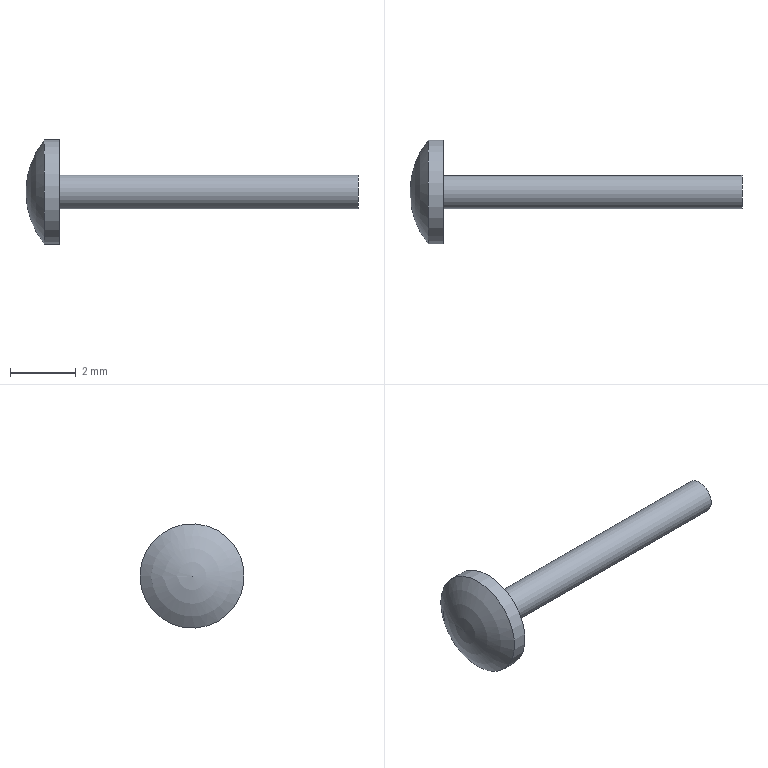Part | NX | features solid 2 | 1 solid | 5 faces | box 10.109 x 3.175 x 3.175 mm | volume 13.301 mm3 | plane 2 | cylinder 2 | sphere 1 | commonest cylinder face diameters 1.016 x1 3.175 x1
STEP:
#1=CARTESIAN_POINT('',(0.,0.508,0.));
#2=VERTEX_POINT('',#1);
#3=CARTESIAN_POINT('',(0.,0.,0.));
#4=DIRECTION('',(1.,0.,0.));
#5=DIRECTION('',(0.,1.,0.));
#6=AXIS2_PLACEMENT_3D('',#3,#4,#5);
#7=CIRCLE('',#6,0.508);
#8=EDGE_CURVE('',#2,#2,#7,.T.);
#9=ORIENTED_EDGE('',*,*,#8,.T.);
#10=EDGE_LOOP('',(#9));
#11=FACE_BOUND('',#10,.T.);
#12=CARTESIAN_POINT('',(0.,0.508,0.));
#13=DIRECTION('',(1.,0.,0.));
#14=DIRECTION('',(0.,1.,0.));
#15=AXIS2_PLACEMENT_3D('',#12,#13,#14);
#16=PLANE('',#15);
#17=ADVANCED_FACE('',(#11),#16,.T.);
#18=CARTESIAN_POINT('',(-9.093,0.508,0.));
#19=VERTEX_POINT('',#18);
#20=CARTESIAN_POINT('',(-9.093,0.,0.));
#21=DIRECTION('',(1.,0.,0.));
#22=DIRECTION('',(0.,1.,0.));
#23=AXIS2_PLACEMENT_3D('',#20,#21,#22);
#24=CIRCLE('',#23,0.508);
#25=EDGE_CURVE('',#19,#19,#24,.T.);
#26=ORIENTED_EDGE('',*,*,#25,.T.);
#27=EDGE_LOOP('',(#26));
#28=FACE_BOUND('',#27,.T.);
#29=ORIENTED_EDGE('',*,*,#8,.F.);
#30=EDGE_LOOP('',(#29));
#31=FACE_BOUND('',#30,.T.);
#32=CARTESIAN_POINT('',(0.,0.,0.));
#33=DIRECTION('',(1.,0.,0.));
#34=DIRECTION('',(0.,1.,0.));
#35=AXIS2_PLACEMENT_3D('',#32,#33,#34);
#36=CYLINDRICAL_SURFACE('',#35,0.508);
#37=ADVANCED_FACE('',(#28,#31),#36,.T.);
#38=CARTESIAN_POINT('',(-9.093,1.587,0.));
#39=VERTEX_POINT('',#38);
#40=CARTESIAN_POINT('',(-9.093,0.,0.));
#41=DIRECTION('',(1.,0.,0.));
#42=DIRECTION('',(0.,1.,0.));
#43=AXIS2_PLACEMENT_3D('',#40,#41,#42);
#44=CIRCLE('',#43,1.587);
#45=EDGE_CURVE('',#39,#39,#44,.T.);
#46=ORIENTED_EDGE('',*,*,#45,.T.);
#47=EDGE_LOOP('',(#46));
#48=FACE_BOUND('',#47,.T.);
#49=ORIENTED_EDGE('',*,*,#25,.F.);
#50=EDGE_LOOP('',(#49));
#51=FACE_BOUND('',#50,.T.);
#52=CARTESIAN_POINT('',(-9.093,1.587,0.));
#53=DIRECTION('',(1.,0.,0.));
#54=DIRECTION('',(0.,1.,0.));
#55=AXIS2_PLACEMENT_3D('',#52,#53,#54);
#56=PLANE('',#55);
#57=ADVANCED_FACE('',(#48,#51),#56,.T.);
#58=CARTESIAN_POINT('',(-9.552,1.587,0.));
#59=VERTEX_POINT('',#58);
#60=CARTESIAN_POINT('',(-9.552,0.,0.));
#61=DIRECTION('',(1.,0.,0.));
#62=DIRECTION('',(0.,1.,0.));
#63=AXIS2_PLACEMENT_3D('',#60,#61,#62);
#64=CIRCLE('',#63,1.587);
#65=EDGE_CURVE('',#59,#59,#64,.T.);
#66=ORIENTED_EDGE('',*,*,#65,.T.);
#67=EDGE_LOOP('',(#66));
#68=FACE_BOUND('',#67,.T.);
#69=ORIENTED_EDGE('',*,*,#45,.F.);
#70=EDGE_LOOP('',(#69));
#71=FACE_BOUND('',#70,.T.);
#72=CARTESIAN_POINT('',(0.,0.,0.));
#73=DIRECTION('',(1.,0.,0.));
#74=DIRECTION('',(0.,1.,0.));
#75=AXIS2_PLACEMENT_3D('',#72,#73,#74);
#76=CYLINDRICAL_SURFACE('',#75,1.587);
#77=ADVANCED_FACE('',(#68,#71),#76,.T.);
#78=ORIENTED_EDGE('',*,*,#65,.F.);
#79=EDGE_LOOP('',(#78));
#80=FACE_BOUND('',#79,.T.);
#81=CARTESIAN_POINT('',(-7.569,0.,0.));
#82=DIRECTION('',(1.,0.,0.));
#83=DIRECTION('',(0.,1.,0.));
#84=AXIS2_PLACEMENT_3D('',#81,#82,#83);
#85=SPHERICAL_SURFACE('',#84,2.54);
#86=ADVANCED_FACE('',(#80),#85,.T.);
#87=CLOSED_SHELL('',(#17,#37,#57,#77,#86));
#88=MANIFOLD_SOLID_BREP('',#87);
#89=(LENGTH_UNIT()NAMED_UNIT(*)SI_UNIT(.MILLI.,.METRE.));
#90=UNCERTAINTY_MEASURE_WITH_UNIT(LENGTH_MEASURE(0.00001),#89,'','');
#91=(NAMED_UNIT(*)PLANE_ANGLE_UNIT()SI_UNIT($,.RADIAN.));
#92=(NAMED_UNIT(*)SI_UNIT($,.STERADIAN.)SOLID_ANGLE_UNIT());
#93=(GEOMETRIC_REPRESENTATION_CONTEXT(3)GLOBAL_UNCERTAINTY_ASSIGNED_CONTEXT((#90))GLOBAL_UNIT_ASSIGNED_CONTEXT((#89,#91,#92))REPRESENTATION_CONTEXT('',''));
#94=ADVANCED_BREP_SHAPE_REPRESENTATION('',(#88),#93);